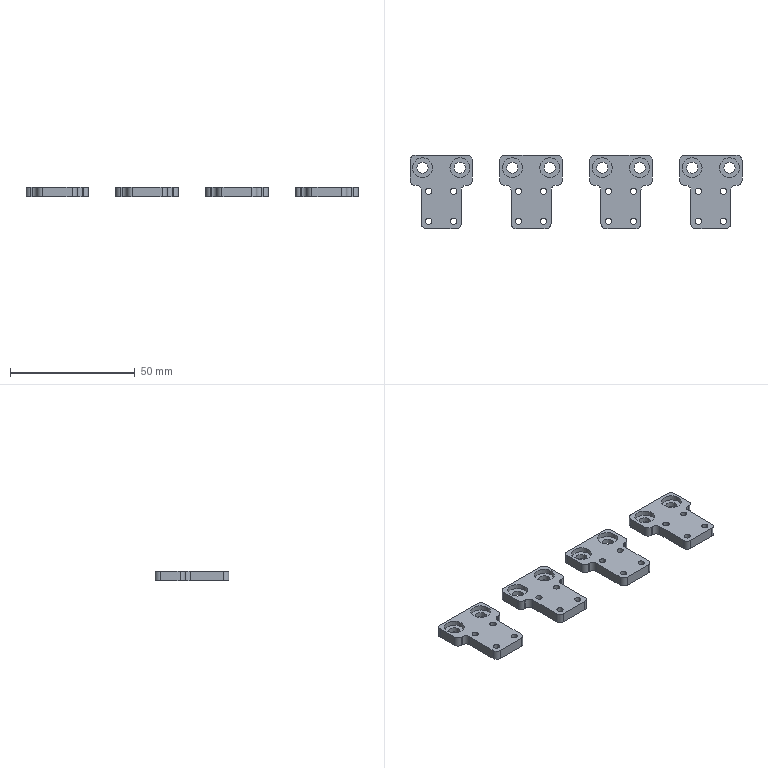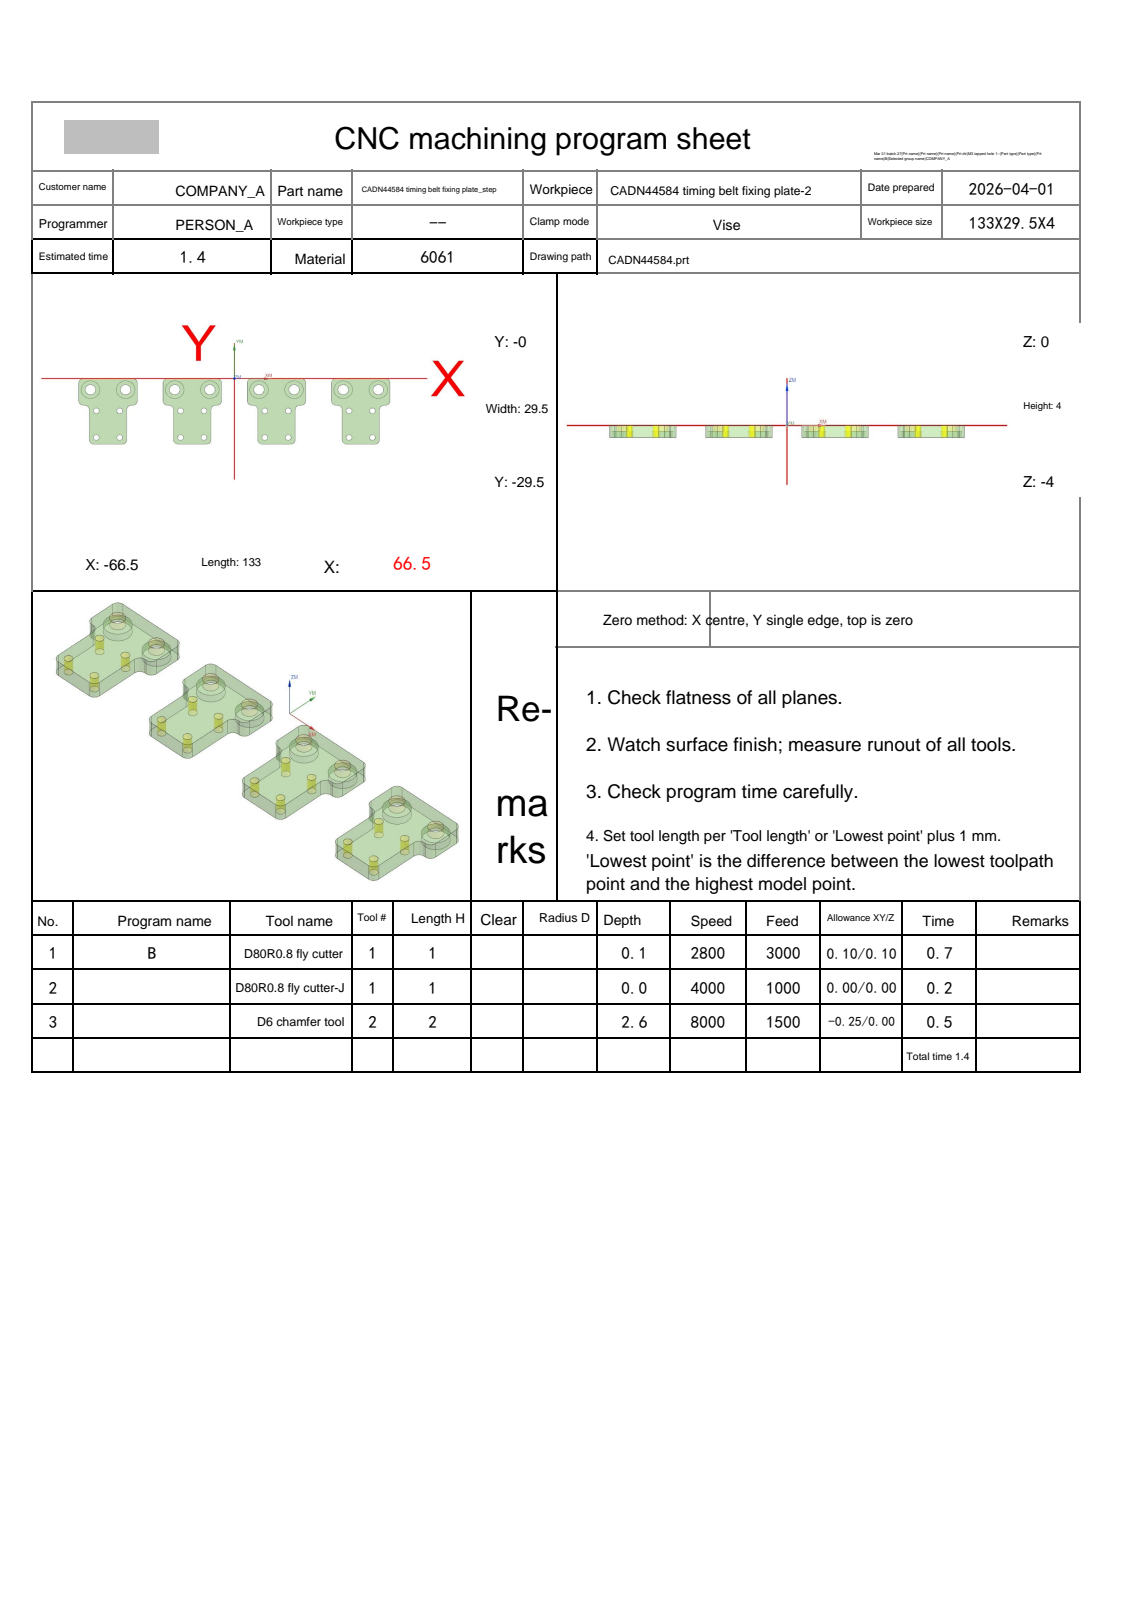NC program | NX | posted by the shop | part box 133 x 29.5 x 4 mm
Whole program:
%
O0001
(Machine time: 2.04 MIN)
(===Total Tool:2===)
(T1=D80R0.8 fly cutter D=80.  R=0.8  D-  H01 Z=0.    )
(T2=D6 chamfer tool   D=6.   R=0.   D-  H02 Z=-2.55 )
G80 G90 G17 G49 G40
G91 G28 Z0
M01
N1 T01 M06
(D80R0.8 fly cutter  D=80. R=0.8 H=01 ce=0.10 di=0.10)
G00 G90 G54 X-118.388 Y-14.75 M03 S2800
G43 H01 Z20.
M08
Z5.014
G01 Z3.014 F3000.
X-106.328
X106.328
X118.388
Z5.014
G00 X-118.388
Z4.529
G01 Z2.529
X-106.328
X106.328
X118.388
Z4.529
G00 X-118.388
Z4.043
G01 Z2.043
X-106.328
X106.328
X118.388
Z4.043
G00 X-118.388
Z3.557
G01 Z1.557
X-106.328
X106.328
X118.388
Z3.557
G00 Z20.
X-118.388
Z3.071
G01 Z1.071
X-106.328
X106.328
X118.388
Z3.071
G00 Z20.
X-118.388
Z2.586
G01 Z.586
X-106.328
X106.328
X118.388
Z2.586
G00 Z20.
X-118.388
Z2.1
G01 Z.1
X-106.328
X106.328
X118.388
Z2.1
G00 Z20.
G91 G28 Z0.0
M05
M09
G91 G28 Z0.0
M01
N2 T01 M06
(D80R0.8 fly cutter-J  D=80. R=0.8 H=01 ce=0.00 di=0.00)
G00 G90 G54 X-118.29 Y-14.75 M03 S4000
G43 H01 Z20.
M08
Z2.
G01 Z0.0 F1000.
X-106.23
X106.23
X118.29
Z2.
G00 Z20.
G91 G28 Z0.0
M05
M09
G91 G28 Z0.0
M01
N3 T02 M06
(D6 chamfer tool  D=6. R=0. H=02 ce=0.00 di=0.00)
G00 G90 G54 X-49. Y-26.5 M03 S8000
G43 H02 Z20.
M08
G98 G81 X-49. Y-26.5 Z-1.75 R3. F1000.
X-59.
Y-14.5
X-49.
X-23.
Y-26.5
X-13.
Y-14.5
X13.
Y-26.5
X23.
Y-14.5
X49.
X59.
Y-26.5
X49.
G80
G00 Z20.
G00 G90 X61.5 Y-5. M03 S8000
Z20.
G98 G81 X61.5 Y-5. Z-2.55 R3. F1000.
X46.5
X25.5
X10.5
X-10.5
X-25.5
X-46.5
X-61.5
G80
G00 Z20.
G00 G90 X41.213 Y-11.523 M03 S7000
Z20.
Z2.5
G01 X41.138 Y-11.413 Z2.452 F1500.
X40.982 Y-11.113 Z2.328
X40.864 Y-10.795 Z2.205
X40.787 Y-10.465 Z2.082
X40.75 Y-10.128 Z1.959
Y-2. Z-1.
G02 X43.5 Y.75 I2.75 J0.0
G01 X64.5
G02 X67.25 Y-2. I0.0 J-2.75
G01 Y-10.
G02 X64.5 Y-12.75 I-2.75 J0.0
G01 X64.
G03 X62.75 Y-14. I0.0 J-1.25
G01 Y-27.5
G02 X60. Y-30.25 I-2.75 J0.0
G01 X48.
G02 X45.25 Y-27.5 I0.0 J2.75
G01 Y-14.
G03 X44. Y-12.75 I-1.25 J0.0
G01 X43.5
G02 X40.75 Y-10. I0.0 J2.75
G01 Y-2.
G02 X40.795 Y-1.503 I2.75 J0.0
G01 Z1.5
G00 Z20.
X5.213 Y-11.523
Z2.5
G01 X5.138 Y-11.413 Z2.452
X4.982 Y-11.113 Z2.328
X4.864 Y-10.795 Z2.205
X4.787 Y-10.465 Z2.082
X4.75 Y-10.128 Z1.959
Y-2. Z-1.
G02 X7.5 Y.75 I2.75 J0.0
G01 X28.5
G02 X31.25 Y-2. I0.0 J-2.75
G01 Y-10.
G02 X28.5 Y-12.75 I-2.75 J0.0
G01 X28.
G03 X26.75 Y-14. I0.0 J-1.25
G01 Y-27.5
G02 X24. Y-30.25 I-2.75 J0.0
G01 X12.
G02 X9.25 Y-27.5 I0.0 J2.75
G01 Y-14.
G03 X8. Y-12.75 I-1.25 J0.0
G01 X7.5
G02 X4.75 Y-10. I0.0 J2.75
G01 Y-2.
G02 X4.795 Y-1.503 I2.75 J0.0
G01 Z1.5
G00 Z20.
X-30.787 Y-11.523
Z2.5
G01 X-30.862 Y-11.413 Z2.452
X-31.018 Y-11.113 Z2.328
X-31.136 Y-10.795 Z2.205
X-31.213 Y-10.465 Z2.082
X-31.25 Y-10.128 Z1.959
Y-2. Z-1.
G02 X-28.5 Y.75 I2.75 J0.0
G01 X-7.5
G02 X-4.75 Y-2. I0.0 J-2.75
G01 Y-10.
G02 X-7.5 Y-12.75 I-2.75 J0.0
G01 X-8.
G03 X-9.25 Y-14. I0.0 J-1.25
G01 Y-27.5
G02 X-12. Y-30.25 I-2.75 J0.0
G01 X-24.
G02 X-26.75 Y-27.5 I0.0 J2.75
G01 Y-14.
G03 X-28. Y-12.75 I-1.25 J0.0
G01 X-28.5
G02 X-31.25 Y-10. I0.0 J2.75
G01 Y-2.
G02 X-31.205 Y-1.503 I2.75 J0.0
G01 Z1.5
G00 Z20.
X-66.787 Y-11.523
Z2.5
G01 X-66.862 Y-11.413 Z2.452
X-67.018 Y-11.113 Z2.328
X-67.136 Y-10.795 Z2.205
X-67.213 Y-10.465 Z2.082
X-67.25 Y-10.128 Z1.959
Y-2. Z-1.
G02 X-64.5 Y.75 I2.75 J0.0
G01 X-43.5
G02 X-40.75 Y-2. I0.0 J-2.75
G01 Y-10.
G02 X-43.5 Y-12.75 I-2.75 J0.0
G01 X-44.
G03 X-45.25 Y-14. I0.0 J-1.25
G01 Y-27.5
G02 X-48. Y-30.25 I-2.75 J0.0
G01 X-60.
G02 X-62.75 Y-27.5 I0.0 J2.75
G01 Y-14.
G03 X-64. Y-12.75 I-1.25 J0.0
G01 X-64.5
G02 X-67.25 Y-10. I0.0 J2.75
G01 Y-2.
G02 X-67.205 Y-1.503 I2.75 J0.0
G01 Z1.5
G00 Z20.
M05
M09
G91 G28 Z0.0
G91 G28 Y0.0
M30
%